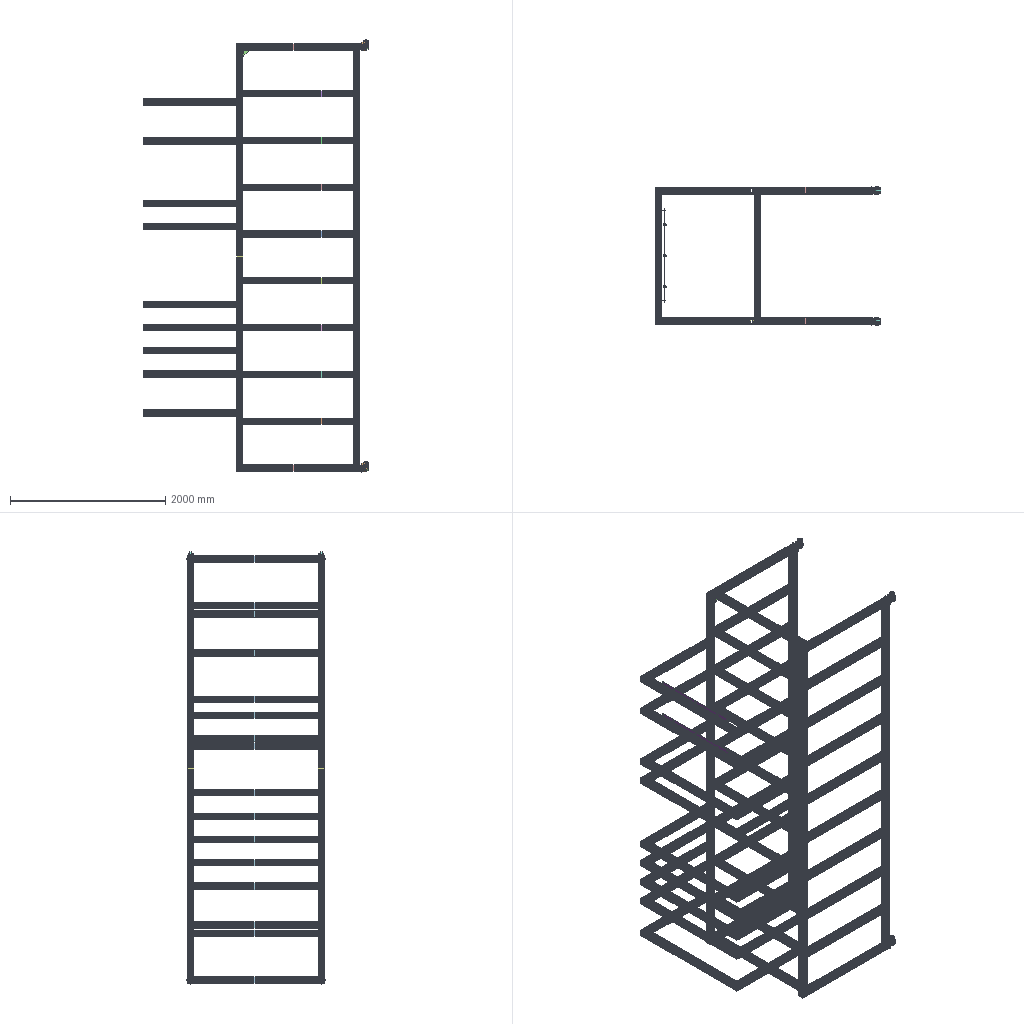Assembly | SolidWorks | 25 different items | 121 placed | box 2901 x 1777 x 5560 mm
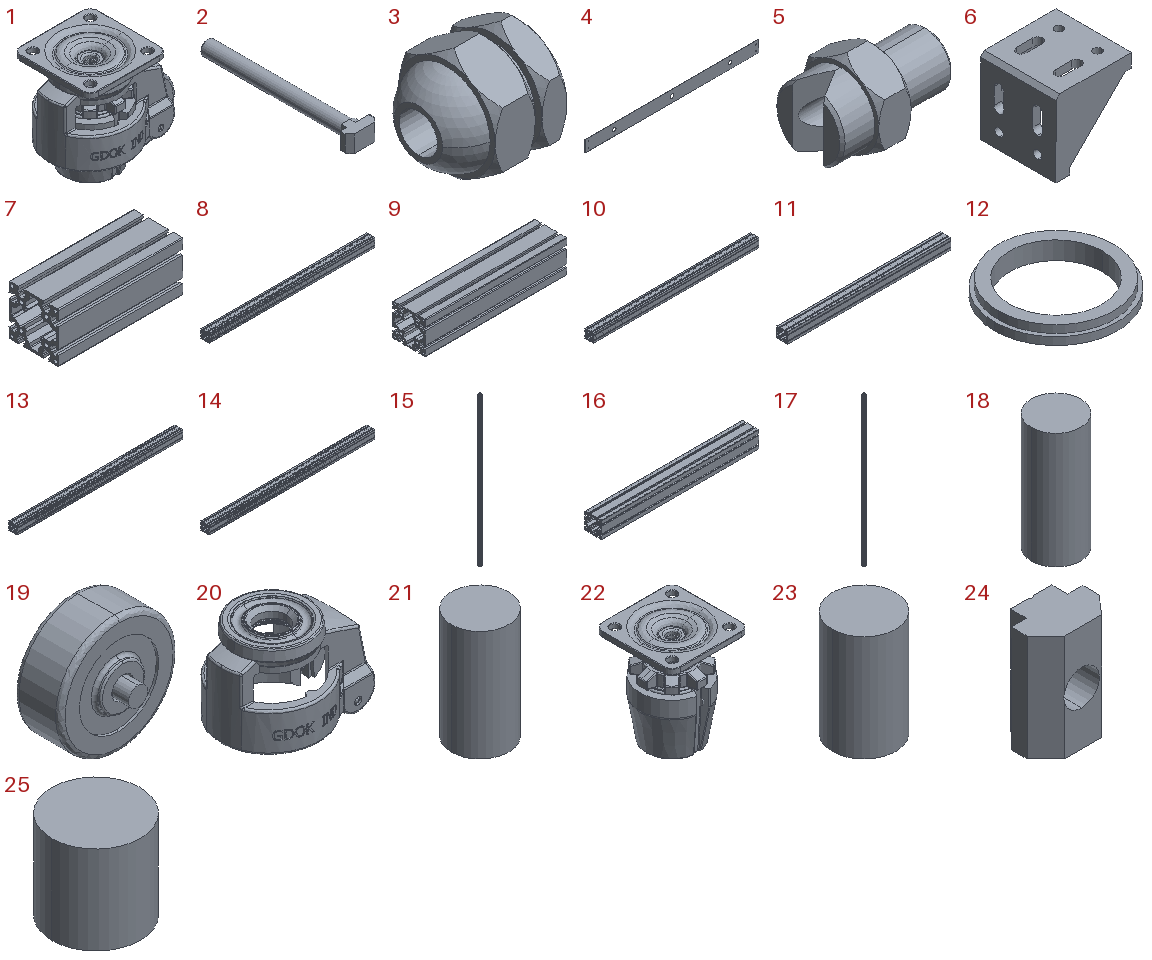Parts list (item | name | quantity | parent item | size | volume | features):
1 | (subassembly) | x4 | - | 141 x 97.04 x 120.76 mm | 659817 mm3 | -
2 | - | x4 | - | 10.5 x 55.3 x 6 mm | 1236 mm3 | features Fillet 2, ICE 2, Chamfer 1, Extrusion 1, Revolution 1
3 | - | x6 | - | 30 x 29 x 33.486 mm | 15189 mm3 | features ICE 4, RevCut 1, Revolution 1
4 | - | x2 | - | 1200 x 2 x 80 mm | 188829 mm3 | features Extrusion 1
5 | - | x6 | - | 22 x 14 x 16.166 mm | 1551 mm3 | features ICE 3, RevCut 1, Revolution 1
6 | - | x1 | - | 78 x 78 x 78 mm | 101387 mm3 | features ICE 11, HoleWzd 2, Chamfer 1, Extrusion 1
7 | - | x1 | - | 200 x 80 x 80 mm | 457804 mm3 | features ICE 1, WeldMemberFeat 1, WeldmentFeature 1
8 | - | x1 | - | 1550 x 80 x 80 mm | 3547982 mm3 | features ICE 1, WeldMemberFeat 1, WeldmentFeature 1
9 | - | x1 | - | 350 x 80 x 80 mm | 801157 mm3 | features ICE 1, WeldMemberFeat 1, WeldmentFeature 1
10 | - | x20 | - | 1500 x 80 x 80 mm | 3433531 mm3 | features ICE 1, WeldMemberFeat 1, WeldmentFeature 1
11 | - | x18 | - | 1200 x 80 x 80 mm | 2746825 mm3 | features ICE 1, WeldMemberFeat 1, WeldmentFeature 1
12 | - | x4 | in 1 | 16 x 16 x 2.338 mm | 153.776 mm3 | features BaseBody 1
13 | - | x9 | - | 1600 x 80 x 80 mm | 3662433 mm3 | features ICE 1, WeldMemberFeat 1, WeldmentFeature 1
14 | - | x10 | - | 1600 x 80 x 80 mm | 3662433 mm3 | features ICE 1, WeldMemberFeat 1, WeldmentFeature 1
15 | - | x2 | - | 80 x 80 x 5338 mm | 9294002 mm3 | features Extrusion 1
16 | - | x1 | - | 750 x 80 x 80 mm | 1716766 mm3 | features ICE 1, WeldMemberFeat 1, WeldmentFeature 1
17 | - | x2 | - | 80 x 80 x 5500 mm | 9576060 mm3 | features Extrusion 1
18 | - | x4 | in 1 | 1 x 1 x 2.34 mm | 1.838 mm3 | features BaseBody 1
19 | - | x4 | in 1 | 74 x 52.5 x 74 mm | 124729 mm3 | features BaseBody 1
20 | - | x4 | in 1 | 122 x 97.04 x 91 mm | 221114 mm3 | features BaseBody 1
21 | - | x4 | in 1 | 2.4 x 2.4 x 4.64 mm | 20.991 mm3 | features BaseBody 1
22 | - | x4 | in 1 | 95 x 95 x 118.5 mm | 311521 mm3 | features BaseBody 1
23 | - | x4 | in 1 | 12 x 12 x 20 mm | 2262 mm3 | features BaseBody 1
24 | - | x1 | - | 13.5 x 9.5 x 20 mm | 1659 mm3 | features BaseBody 1
25 | - | x4 | in 1 | 1 x 1 x 1 mm | 0.7854 mm3 | features BaseBody 1
Mates (type | each side: item.copy, entity, surface, feature):
Coincident | 10.1 face plane Aluminium profile 80 X 80G X R1.5(1) | 22.1 face plane Input1
Concentric | 10.1 face cylinder Aluminium profile 80 X 80G X R1.5(1) | 22.1 face cylinder Input1
Concentric | 10.1 face cylinder Cut-Extrude1 | 22.1 face cylinder Input1
Coincident | 10.1 face plane Aluminium profile 80 X 80G X R1.5(1) | 14.1 face plane Aluminium profile 80 X 80G X R1.5(1) | 3 times
Coincident | 10.1 face plane Aluminium profile 80 X 80G X R1.5(1) | 17.1 face plane Boss-Extrude1 | 3 times
Coincident | 10.2 face plane Aluminium profile 80 X 80G X R1.5(1) | 15.1 face plane Boss-Extrude1 | 3 times
Coincident | 10.2 face plane Aluminium profile 80 X 80G X R1.5(1) | 6.1 face plane Boss-Extrude2
Coincident | 17.2 face plane Boss-Extrude1 | 6.1 face plane Boss-Extrude4
Coincident | 10.2 face plane Aluminium profile 80 X 80G X R1.5(1) | 6.1 face plane Boss-Extrude1
Coincident | 17.2 face plane Boss-Extrude1 | 11.1 face plane Aluminium profile 80 X 80G X R1.5(1) | 2 times
DistanceDim | 11.1 face plane Aluminium profile 80 X 80G X R1.5(1) | 17.2 face plane Boss-Extrude1
Coincident | 17.2 face plane Boss-Extrude1 | 11.2 face plane Aluminium profile 80 X 80G X R1.5(1)
Coincident | 17.1 face plane Boss-Extrude1 | 11.2 face plane Aluminium profile 80 X 80G X R1.5(1)
DistanceDim | 11.2 face plane Aluminium profile 80 X 80G X R1.5(1) | 17.2 face plane Boss-Extrude1
Coincident | 11.2 face plane Aluminium profile 80 X 80G X R1.5(1) | 13.1 face plane Aluminium profile 80 X 80G X R1.5(1) | 3 times
Coincident | 13.1 face plane Aluminium profile 80 X 80G X R1.5(1) | 2.1 face plane Cut-Extrude1
Symmetric | 13.1 face plane Aluminium profile 80 X 80G X R1.5(1) | 13.1 face plane Aluminium profile 80 X 80G X R1.5(1) | 2.1 plane
Concentric | 5.1 face cylinder Revolve1 | 3.1 face cylinder Revolve1
Coincident | 5.1 face plane Revolve1 | 3.1 face plane Revolve1
Concentric | 4.1 face cylinder Boss-Extrude1 | 3.1 face cylinder Revolve1
Coincident | 4.1 face plane Boss-Extrude1 | 3.1 face plane Revolve1
DistanceDim | 13.1 face plane Aluminium profile 80 X 80G X R1.5(1) | 2.1 face plane Boss-Extrude1
Concentric | 2.1 face cylinder Revolve1 | 4.1 face cylinder Boss-Extrude1
Concentric | 2.2 face cylinder Revolve1 | 4.1 face cylinder Boss-Extrude1
DistanceDim | 3.1 face plane Revolve1 | 13.1 face plane Aluminium profile 80 X 80G X R1.5(1)